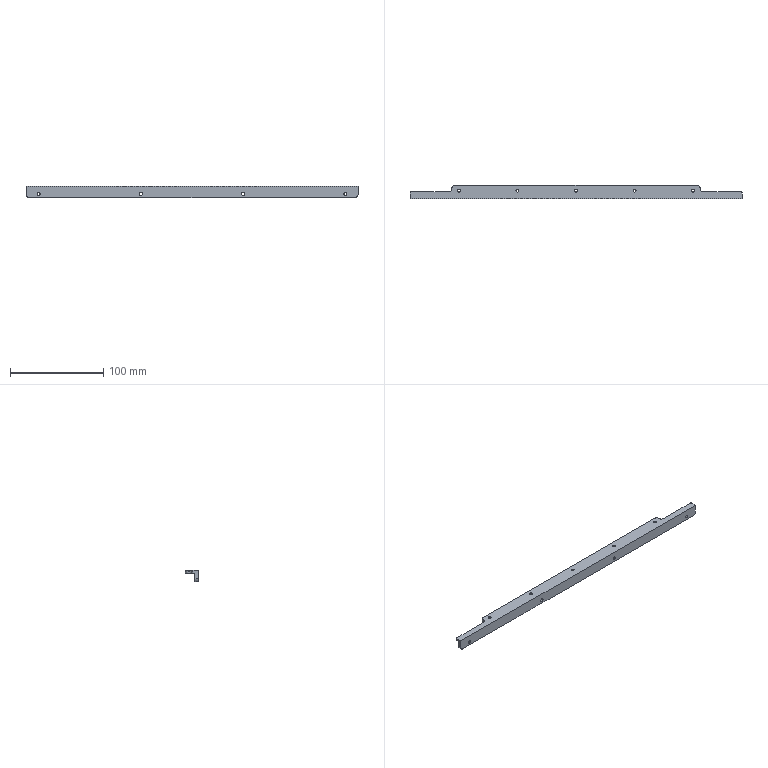NC program | NX | posted with a generic post | part box 356.96 x 14 x 12 mm
Whole program:
N10 G17 G21 G94 G90
(PLANAR_MILL_3 , TOOL : D16精光)
N12 T06 M6
N14 G54
N16 G17 G0 G90 X191.48 Y-0.001 B0. C0. S4500 M3
N18 G43 Z30. H6
N20 Z4.517
N22 G94 G1 Z2.517 F1200.
N24 X178.48
N26 X-178.48
N28 X-191.48
N30 Z4.517
N32 G0 Z30.
N34 X191.48
N36 Z4.033
N38 G1 Z2.033
N40 X178.48
N42 X-178.48
N44 X-191.48
N46 Z4.033
N48 G0 Z30.
N50 X191.48
N52 Z3.55
N54 G1 Z1.55
N56 X178.48
N58 X-178.48
N60 X-191.48
N62 Z3.55
N64 G0 Z30.
N66 X191.48
N68 Z3.067
N70 G1 Z1.067
N72 X178.48
N74 X-178.48
N76 X-191.48
N78 Z3.067
N80 G0 Z30.
N82 X191.48
N84 Z2.583
N86 G1 Z0.583
N88 X178.48
N90 X-178.48
N92 X-191.48
N94 Z2.583
N96 G0 Z30.
N98 X191.48
N100 Z2.1
N102 G1 Z0.1
N104 X178.48
N106 X-178.48
N108 X-191.48
N110 Z2.1
N112 G0 Z30.
(PLANAR_MILL_3_COPY , TOOL : D16精光)
N114 X191.48
N116 Z2.
N118 G1 Z0. F800.
N120 X178.48
N122 X-178.48
N124 X-191.48
N126 Z2.
N128 G0 Z30.
N130 M5
(PLANAR_MILL_4 , TOOL : D6点钻)
N132 T03 M6
N134 G54
N136 G17 G0 G90 X181.308 Y-8.001 B0. C0. S3500 M3
N138 G43 Z30. H3
N140 Z1.
N142 G94 G1 Z-1. F1000.
N144 X178.479
N146 X-178.48
N148 G2 X-179.48 Y-7.001 R1.
N150 G1 Y-1.001
N152 G2 X-177.48 Y0.999 R2.
N154 G1 X-136.5
N156 G3 X-134.5 Y2.999 R2.
N158 G1 Y3.999
N160 G2 X-130.5 Y7.999 R4.
N162 G1 X130.5
N164 G2 X134.5 Y3.999 R4.
N166 G1 Y2.999
N168 G3 X136.5 Y0.999 R2.
N170 G1 X177.48
N172 G2 X179.48 Y-1.001 R2.
N174 G1 Y-7.
N176 Y-9.83
N178 Z1.
N180 G0 Z30.
(DRILLING_1 , TOOL : D6点钻)
N182 X-126. Y1.499 S3000
N184 G81 G98 Z-1.6 F300. R3.
N186 X-63.
N188 X0.
N190 X63.
N192 X126.
N194 G80
N196 G0 X126. Y1.499 Z30.
N198 M5
N200 M2